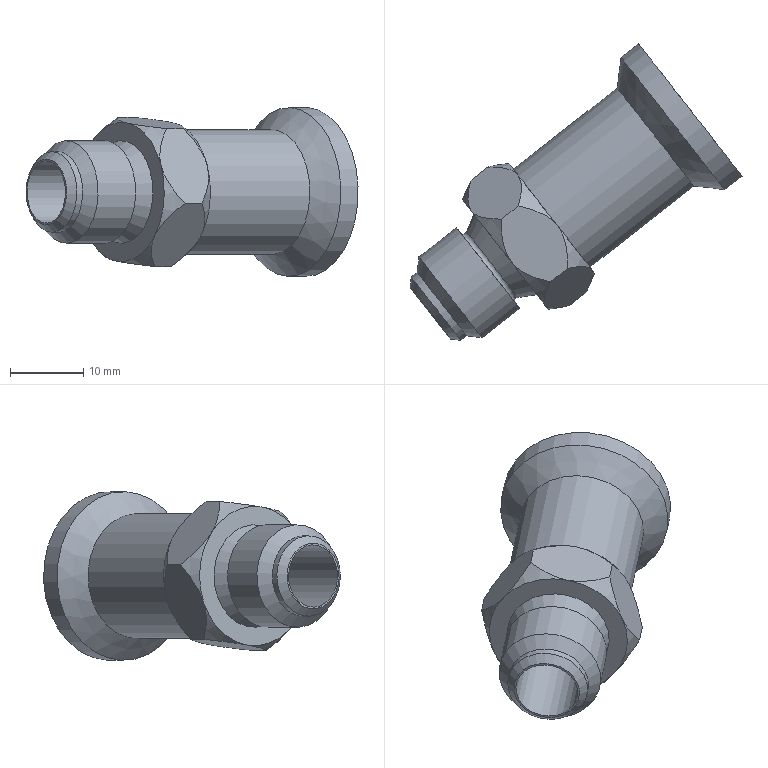Part | NX | features BREP 1 | 1 solid | 35 faces | box 45.311 x 40.485 x 23 mm | volume 6517 mm3 | cone 17 | plane 11 | cylinder 6 | torus 1 | commonest cylinder face diameters 8.5 x1 11 x1 12.5 x1 14 x1 17 x1 23 x1
STEP:
#1=CARTESIAN_POINT('',(-0.7107,91.095,-108.342));
#2=VERTEX_POINT('',#1);
#3=CARTESIAN_POINT('',(-6.134,98.036,-111.901));
#4=VERTEX_POINT('',#3);
#5=CARTESIAN_POINT('',(-1.525,92.137,-117.75));
#6=DIRECTION('',(-0.788,-0.6157,0.));
#7=DIRECTION('',(0.379,-0.4851,0.788));
#8=AXIS2_PLACEMENT_3D('',#5,#6,#7);
#9=CIRCLE('',#8,9.5);
#10=EDGE_CURVE('',#2,#4,#9,.T.);
#11=ORIENTED_EDGE('',*,*,#10,.F.);
#12=CARTESIAN_POINT('',(3.898,85.196,-114.191));
#13=VERTEX_POINT('',#12);
#14=CARTESIAN_POINT('',(-1.525,92.137,-117.75));
#15=DIRECTION('',(-0.788,-0.6157,0.));
#16=DIRECTION('',(0.379,-0.4851,0.788));
#17=AXIS2_PLACEMENT_3D('',#14,#15,#16);
#18=CIRCLE('',#17,9.5);
#19=EDGE_CURVE('',#13,#2,#18,.T.);
#20=ORIENTED_EDGE('',*,*,#19,.F.);
#21=CARTESIAN_POINT('',(3.084,86.238,-123.599));
#22=VERTEX_POINT('',#21);
#23=CARTESIAN_POINT('',(-1.525,92.137,-117.75));
#24=DIRECTION('',(-0.788,-0.6157,0.));
#25=DIRECTION('',(0.379,-0.4851,0.788));
#26=AXIS2_PLACEMENT_3D('',#23,#24,#25);
#27=CIRCLE('',#26,9.5);
#28=EDGE_CURVE('',#22,#13,#27,.T.);
#29=ORIENTED_EDGE('',*,*,#28,.F.);
#30=CARTESIAN_POINT('',(-2.339,93.179,-127.158));
#31=VERTEX_POINT('',#30);
#32=CARTESIAN_POINT('',(-1.525,92.137,-117.75));
#33=DIRECTION('',(-0.788,-0.6157,0.));
#34=DIRECTION('',(0.379,-0.4851,0.788));
#35=AXIS2_PLACEMENT_3D('',#32,#33,#34);
#36=CIRCLE('',#35,9.5);
#37=EDGE_CURVE('',#31,#22,#36,.T.);
#38=ORIENTED_EDGE('',*,*,#37,.F.);
#39=CARTESIAN_POINT('',(-6.948,99.078,-121.309));
#40=VERTEX_POINT('',#39);
#41=CARTESIAN_POINT('',(-1.525,92.137,-117.75));
#42=DIRECTION('',(-0.788,-0.6157,0.));
#43=DIRECTION('',(0.379,-0.4851,0.788));
#44=AXIS2_PLACEMENT_3D('',#41,#42,#43);
#45=CIRCLE('',#44,9.5);
#46=EDGE_CURVE('',#40,#31,#45,.T.);
#47=ORIENTED_EDGE('',*,*,#46,.F.);
#48=CARTESIAN_POINT('',(-1.525,92.137,-117.75));
#49=DIRECTION('',(0.788,0.6157,0.));
#50=DIRECTION('',(-0.379,0.4851,-0.788));
#51=AXIS2_PLACEMENT_3D('',#48,#49,#50);
#52=CIRCLE('',#51,9.5);
#53=EDGE_CURVE('',#40,#4,#52,.T.);
#54=ORIENTED_EDGE('',*,*,#53,.T.);
#55=EDGE_LOOP('',(#11,#20,#29,#38,#47,#54));
#56=FACE_BOUND('',#55,.T.);
#57=CARTESIAN_POINT('',(1.697,88.013,-111.052));
#58=VERTEX_POINT('',#57);
#59=CARTESIAN_POINT('',(-1.525,92.137,-117.75));
#60=DIRECTION('',(0.788,0.6157,0.));
#61=DIRECTION('',(0.379,-0.4851,0.788));
#62=AXIS2_PLACEMENT_3D('',#59,#60,#61);
#63=CIRCLE('',#62,8.5);
#64=EDGE_CURVE('',#58,#58,#63,.T.);
#65=ORIENTED_EDGE('',*,*,#64,.F.);
#66=EDGE_LOOP('',(#65));
#67=FACE_BOUND('',#66,.T.);
#68=CARTESIAN_POINT('',(0.1033,90.053,-98.935));
#69=DIRECTION('',(-0.788,-0.6157,0.));
#70=DIRECTION('',(-0.379,0.4851,-0.788));
#71=AXIS2_PLACEMENT_3D('',#68,#69,#70);
#72=PLANE('',#71);
#73=ADVANCED_FACE('',(#56,#67),#72,.F.);
#74=CARTESIAN_POINT('',(-2.406,80.271,-114.191));
#75=VERTEX_POINT('',#74);
#76=CARTESIAN_POINT('',(-7.015,86.17,-108.342));
#77=VERTEX_POINT('',#76);
#78=CARTESIAN_POINT('',(-7.829,87.212,-117.75));
#79=DIRECTION('',(-0.788,-0.6157,0.));
#80=DIRECTION('',(0.379,-0.4851,0.788));
#81=AXIS2_PLACEMENT_3D('',#78,#79,#80);
#82=CIRCLE('',#81,9.5);
#83=EDGE_CURVE('',#75,#77,#82,.T.);
#84=ORIENTED_EDGE('',*,*,#83,.T.);
#85=CARTESIAN_POINT('',(-12.438,93.111,-111.901));
#86=VERTEX_POINT('',#85);
#87=CARTESIAN_POINT('',(-7.829,87.212,-117.75));
#88=DIRECTION('',(-0.788,-0.6157,0.));
#89=DIRECTION('',(0.379,-0.4851,0.788));
#90=AXIS2_PLACEMENT_3D('',#87,#88,#89);
#91=CIRCLE('',#90,9.5);
#92=EDGE_CURVE('',#77,#86,#91,.T.);
#93=ORIENTED_EDGE('',*,*,#92,.T.);
#94=CARTESIAN_POINT('',(-13.252,94.153,-121.309));
#95=VERTEX_POINT('',#94);
#96=CARTESIAN_POINT('',(-7.829,87.212,-117.75));
#97=DIRECTION('',(-0.788,-0.6157,0.));
#98=DIRECTION('',(0.379,-0.4851,0.788));
#99=AXIS2_PLACEMENT_3D('',#96,#97,#98);
#100=CIRCLE('',#99,9.5);
#101=EDGE_CURVE('',#86,#95,#100,.T.);
#102=ORIENTED_EDGE('',*,*,#101,.T.);
#103=CARTESIAN_POINT('',(-8.643,88.254,-127.158));
#104=VERTEX_POINT('',#103);
#105=CARTESIAN_POINT('',(-7.829,87.212,-117.75));
#106=DIRECTION('',(-0.788,-0.6157,0.));
#107=DIRECTION('',(0.379,-0.4851,0.788));
#108=AXIS2_PLACEMENT_3D('',#105,#106,#107);
#109=CIRCLE('',#108,9.5);
#110=EDGE_CURVE('',#95,#104,#109,.T.);
#111=ORIENTED_EDGE('',*,*,#110,.T.);
#112=CARTESIAN_POINT('',(-3.22,81.313,-123.599));
#113=VERTEX_POINT('',#112);
#114=CARTESIAN_POINT('',(-7.829,87.212,-117.75));
#115=DIRECTION('',(-0.788,-0.6157,0.));
#116=DIRECTION('',(0.379,-0.4851,0.788));
#117=AXIS2_PLACEMENT_3D('',#114,#115,#116);
#118=CIRCLE('',#117,9.5);
#119=EDGE_CURVE('',#104,#113,#118,.T.);
#120=ORIENTED_EDGE('',*,*,#119,.T.);
#121=CARTESIAN_POINT('',(-7.829,87.212,-117.75));
#122=DIRECTION('',(-0.788,-0.6157,0.));
#123=DIRECTION('',(0.379,-0.4851,0.788));
#124=AXIS2_PLACEMENT_3D('',#121,#122,#123);
#125=CIRCLE('',#124,9.5);
#126=EDGE_CURVE('',#113,#75,#125,.T.);
#127=ORIENTED_EDGE('',*,*,#126,.T.);
#128=EDGE_LOOP('',(#84,#93,#102,#111,#120,#127));
#129=FACE_BOUND('',#128,.T.);
#130=CARTESIAN_POINT('',(-10.482,90.608,-123.266));
#131=VERTEX_POINT('',#130);
#132=CARTESIAN_POINT('',(-7.829,87.212,-117.75));
#133=DIRECTION('',(0.788,0.6157,0.));
#134=DIRECTION('',(-0.379,0.4851,-0.788));
#135=AXIS2_PLACEMENT_3D('',#132,#133,#134);
#136=CIRCLE('',#135,7.);
#137=EDGE_CURVE('',#131,#131,#136,.T.);
#138=ORIENTED_EDGE('',*,*,#137,.T.);
#139=EDGE_LOOP('',(#138));
#140=FACE_BOUND('',#139,.T.);
#141=CARTESIAN_POINT('',(-6.201,85.128,-98.935));
#142=DIRECTION('',(-0.788,-0.6157,0.));
#143=DIRECTION('',(-0.379,0.4851,-0.788));
#144=AXIS2_PLACEMENT_3D('',#141,#142,#143);
#145=PLANE('',#144);
#146=ADVANCED_FACE('',(#129,#140),#145,.T.);
#147=CARTESIAN_POINT('',(0.865,80.219,-119.277));
#148=VERTEX_POINT('',#147);
#149=CARTESIAN_POINT('',(0.865,80.219,-119.277));
#150=CARTESIAN_POINT('',(0.1526,80.033,-118.553));
#151=CARTESIAN_POINT('',(-1.199,79.757,-117.033));
#152=CARTESIAN_POINT('',(-2.165,79.963,-115.158));
#153=CARTESIAN_POINT('',(-2.406,80.271,-114.191));
#154=B_SPLINE_CURVE_WITH_KNOTS('',3,(#149,#150,#151,#152,#153),.UNSPECIFIED.,.F.,.F.,(4,1,4),(0.,0.003069,0.006138),.UNSPECIFIED.);
#155=EDGE_CURVE('',#148,#75,#154,.T.);
#156=ORIENTED_EDGE('',*,*,#155,.F.);
#157=CARTESIAN_POINT('',(3.157,82.01,-119.277));
#158=VERTEX_POINT('',#157);
#159=CARTESIAN_POINT('',(-1.141,78.652,-119.277));
#160=DIRECTION('',(0.788,0.6157,0.));
#161=VECTOR('',#160,1000.);
#162=LINE('',#159,#161);
#163=EDGE_CURVE('',#148,#158,#162,.T.);
#164=ORIENTED_EDGE('',*,*,#163,.T.);
#165=CARTESIAN_POINT('',(3.898,85.196,-114.191));
#166=CARTESIAN_POINT('',(4.139,84.888,-115.159));
#167=CARTESIAN_POINT('',(4.107,83.91,-117.018));
#168=CARTESIAN_POINT('',(3.51,82.657,-118.552));
#169=CARTESIAN_POINT('',(3.157,82.01,-119.277));
#170=B_SPLINE_CURVE_WITH_KNOTS('',3,(#165,#166,#167,#168,#169),.UNSPECIFIED.,.F.,.F.,(4,1,4),(0.,0.003072,0.006144),.UNSPECIFIED.);
#171=EDGE_CURVE('',#13,#158,#170,.T.);
#172=ORIENTED_EDGE('',*,*,#171,.F.);
#173=CARTESIAN_POINT('',(0.6273,85.248,-109.106));
#174=VERTEX_POINT('',#173);
#175=CARTESIAN_POINT('',(0.6273,85.248,-109.106));
#176=CARTESIAN_POINT('',(1.34,85.434,-109.829));
#177=CARTESIAN_POINT('',(2.691,85.71,-111.35));
#178=CARTESIAN_POINT('',(3.658,85.504,-113.224));
#179=CARTESIAN_POINT('',(3.898,85.196,-114.191));
#180=B_SPLINE_CURVE_WITH_KNOTS('',3,(#175,#176,#177,#178,#179),.UNSPECIFIED.,.F.,.F.,(4,1,4),(0.,0.003069,0.006138),.UNSPECIFIED.);
#181=EDGE_CURVE('',#174,#13,#180,.T.);
#182=ORIENTED_EDGE('',*,*,#181,.F.);
#183=CARTESIAN_POINT('',(-1.665,83.457,-109.106));
#184=VERTEX_POINT('',#183);
#185=CARTESIAN_POINT('',(-3.671,81.89,-109.106));
#186=DIRECTION('',(0.788,0.6157,0.));
#187=VECTOR('',#186,1000.);
#188=LINE('',#185,#187);
#189=EDGE_CURVE('',#184,#174,#188,.T.);
#190=ORIENTED_EDGE('',*,*,#189,.F.);
#191=CARTESIAN_POINT('',(-2.406,80.271,-114.191));
#192=CARTESIAN_POINT('',(-2.647,80.579,-113.224));
#193=CARTESIAN_POINT('',(-2.615,81.557,-111.365));
#194=CARTESIAN_POINT('',(-2.018,82.81,-109.83));
#195=CARTESIAN_POINT('',(-1.665,83.457,-109.106));
#196=B_SPLINE_CURVE_WITH_KNOTS('',3,(#191,#192,#193,#194,#195),.UNSPECIFIED.,.F.,.F.,(4,1,4),(0.,0.003072,0.006144),.UNSPECIFIED.);
#197=EDGE_CURVE('',#75,#184,#196,.T.);
#198=ORIENTED_EDGE('',*,*,#197,.F.);
#199=EDGE_LOOP('',(#156,#164,#172,#182,#190,#198));
#200=FACE_BOUND('',#199,.T.);
#201=CARTESIAN_POINT('',(-1.141,78.652,-119.277));
#202=DIRECTION('',(-0.5708,0.7306,-0.3746));
#203=DIRECTION('',(-0.2306,0.2952,0.9272));
#204=AXIS2_PLACEMENT_3D('',#201,#202,#203);
#205=PLANE('',#204);
#206=ADVANCED_FACE('',(#200),#205,.F.);
#207=CARTESIAN_POINT('',(-1.665,83.457,-109.106));
#208=CARTESIAN_POINT('',(-2.673,83.65,-108.997));
#209=CARTESIAN_POINT('',(-4.646,84.169,-108.769));
#210=CARTESIAN_POINT('',(-6.379,85.356,-108.488));
#211=CARTESIAN_POINT('',(-7.015,86.17,-108.342));
#212=B_SPLINE_CURVE_WITH_KNOTS('',3,(#207,#208,#209,#210,#211),.UNSPECIFIED.,.F.,.F.,(4,1,4),(0.,0.003069,0.006138),.UNSPECIFIED.);
#213=EDGE_CURVE('',#184,#77,#212,.T.);
#214=ORIENTED_EDGE('',*,*,#213,.F.);
#215=ORIENTED_EDGE('',*,*,#189,.T.);
#216=CARTESIAN_POINT('',(-0.7107,91.095,-108.342));
#217=CARTESIAN_POINT('',(-0.0745,90.281,-108.488));
#218=CARTESIAN_POINT('',(0.6537,88.33,-108.767));
#219=CARTESIAN_POINT('',(0.6842,86.274,-108.997));
#220=CARTESIAN_POINT('',(0.6273,85.248,-109.106));
#221=B_SPLINE_CURVE_WITH_KNOTS('',3,(#216,#217,#218,#219,#220),.UNSPECIFIED.,.F.,.F.,(4,1,4),(0.,0.003072,0.006144),.UNSPECIFIED.);
#222=EDGE_CURVE('',#2,#174,#221,.T.);
#223=ORIENTED_EDGE('',*,*,#222,.F.);
#224=CARTESIAN_POINT('',(-6.061,93.808,-107.579));
#225=VERTEX_POINT('',#224);
#226=CARTESIAN_POINT('',(-6.061,93.808,-107.579));
#227=CARTESIAN_POINT('',(-5.053,93.615,-107.688));
#228=CARTESIAN_POINT('',(-3.079,93.096,-107.916));
#229=CARTESIAN_POINT('',(-1.347,91.909,-108.197));
#230=CARTESIAN_POINT('',(-0.7107,91.095,-108.342));
#231=B_SPLINE_CURVE_WITH_KNOTS('',3,(#226,#227,#228,#229,#230),.UNSPECIFIED.,.F.,.F.,(4,1,4),(0.,0.003069,0.006138),.UNSPECIFIED.);
#232=EDGE_CURVE('',#225,#2,#231,.T.);
#233=ORIENTED_EDGE('',*,*,#232,.F.);
#234=CARTESIAN_POINT('',(-8.353,92.017,-107.579));
#235=VERTEX_POINT('',#234);
#236=CARTESIAN_POINT('',(-10.359,90.45,-107.579));
#237=DIRECTION('',(0.788,0.6157,0.));
#238=VECTOR('',#237,1000.);
#239=LINE('',#236,#238);
#240=EDGE_CURVE('',#235,#225,#239,.T.);
#241=ORIENTED_EDGE('',*,*,#240,.F.);
#242=CARTESIAN_POINT('',(-7.015,86.17,-108.342));
#243=CARTESIAN_POINT('',(-7.651,86.984,-108.197));
#244=CARTESIAN_POINT('',(-8.379,88.935,-107.918));
#245=CARTESIAN_POINT('',(-8.41,90.991,-107.688));
#246=CARTESIAN_POINT('',(-8.353,92.017,-107.579));
#247=B_SPLINE_CURVE_WITH_KNOTS('',3,(#242,#243,#244,#245,#246),.UNSPECIFIED.,.F.,.F.,(4,1,4),(0.,0.003072,0.006144),.UNSPECIFIED.);
#248=EDGE_CURVE('',#77,#235,#247,.T.);
#249=ORIENTED_EDGE('',*,*,#248,.F.);
#250=EDGE_LOOP('',(#214,#215,#223,#233,#241,#249));
#251=FACE_BOUND('',#250,.T.);
#252=CARTESIAN_POINT('',(-3.671,81.89,-109.106));
#253=DIRECTION('',(-0.08568,0.1097,-0.9903));
#254=DIRECTION('',(-0.6097,0.7803,0.1392));
#255=AXIS2_PLACEMENT_3D('',#252,#253,#254);
#256=PLANE('',#255);
#257=ADVANCED_FACE('',(#251),#256,.F.);
#258=CARTESIAN_POINT('',(-8.353,92.017,-107.579));
#259=CARTESIAN_POINT('',(-9.181,91.98,-108.194));
#260=CARTESIAN_POINT('',(-10.776,92.015,-109.486));
#261=CARTESIAN_POINT('',(-12.042,92.605,-111.079));
#262=CARTESIAN_POINT('',(-12.438,93.111,-111.901));
#263=B_SPLINE_CURVE_WITH_KNOTS('',3,(#258,#259,#260,#261,#262),.UNSPECIFIED.,.F.,.F.,(4,1,4),(0.,0.003069,0.006138),.UNSPECIFIED.);
#264=EDGE_CURVE('',#235,#86,#263,.T.);
#265=ORIENTED_EDGE('',*,*,#264,.F.);
#266=ORIENTED_EDGE('',*,*,#240,.T.);
#267=CARTESIAN_POINT('',(-6.134,98.036,-111.901));
#268=CARTESIAN_POINT('',(-5.738,97.53,-111.079));
#269=CARTESIAN_POINT('',(-5.472,96.171,-109.499));
#270=CARTESIAN_POINT('',(-5.823,94.604,-108.195));
#271=CARTESIAN_POINT('',(-6.061,93.808,-107.579));
#272=B_SPLINE_CURVE_WITH_KNOTS('',3,(#267,#268,#269,#270,#271),.UNSPECIFIED.,.F.,.F.,(4,1,4),(0.,0.003072,0.006144),.UNSPECIFIED.);
#273=EDGE_CURVE('',#4,#225,#272,.T.);
#274=ORIENTED_EDGE('',*,*,#273,.F.);
#275=CARTESIAN_POINT('',(-10.218,99.13,-116.223));
#276=VERTEX_POINT('',#275);
#277=CARTESIAN_POINT('',(-10.218,99.13,-116.223));
#278=CARTESIAN_POINT('',(-9.39,99.167,-115.609));
#279=CARTESIAN_POINT('',(-7.796,99.132,-114.316));
#280=CARTESIAN_POINT('',(-6.529,98.542,-112.723));
#281=CARTESIAN_POINT('',(-6.134,98.036,-111.901));
#282=B_SPLINE_CURVE_WITH_KNOTS('',3,(#277,#278,#279,#280,#281),.UNSPECIFIED.,.F.,.F.,(4,1,4),(0.,0.003069,0.006138),.UNSPECIFIED.);
#283=EDGE_CURVE('',#276,#4,#282,.T.);
#284=ORIENTED_EDGE('',*,*,#283,.F.);
#285=CARTESIAN_POINT('',(-12.511,97.339,-116.223));
#286=VERTEX_POINT('',#285);
#287=CARTESIAN_POINT('',(-14.517,95.772,-116.223));
#288=DIRECTION('',(0.788,0.6157,0.));
#289=VECTOR('',#288,1000.);
#290=LINE('',#287,#289);
#291=EDGE_CURVE('',#286,#276,#290,.T.);
#292=ORIENTED_EDGE('',*,*,#291,.F.);
#293=CARTESIAN_POINT('',(-12.438,93.111,-111.901));
#294=CARTESIAN_POINT('',(-12.833,93.617,-112.724));
#295=CARTESIAN_POINT('',(-13.099,94.976,-114.303));
#296=CARTESIAN_POINT('',(-12.748,96.543,-115.608));
#297=CARTESIAN_POINT('',(-12.511,97.339,-116.223));
#298=B_SPLINE_CURVE_WITH_KNOTS('',3,(#293,#294,#295,#296,#297),.UNSPECIFIED.,.F.,.F.,(4,1,4),(0.,0.003072,0.006144),.UNSPECIFIED.);
#299=EDGE_CURVE('',#86,#286,#298,.T.);
#300=ORIENTED_EDGE('',*,*,#299,.F.);
#301=EDGE_LOOP('',(#265,#266,#274,#284,#292,#300));
#302=FACE_BOUND('',#301,.T.);
#303=CARTESIAN_POINT('',(-10.359,90.45,-107.579));
#304=DIRECTION('',(0.4851,-0.621,-0.6157));
#305=DIRECTION('',(-0.788,-0.6157,0.));
#306=AXIS2_PLACEMENT_3D('',#303,#304,#305);
#307=PLANE('',#306);
#308=ADVANCED_FACE('',(#302),#307,.F.);
#309=CARTESIAN_POINT('',(-12.511,97.339,-116.223));
#310=CARTESIAN_POINT('',(-12.863,96.693,-116.947));
#311=CARTESIAN_POINT('',(-13.458,95.448,-118.467));
#312=CARTESIAN_POINT('',(-13.492,94.461,-120.342));
#313=CARTESIAN_POINT('',(-13.252,94.153,-121.309));
#314=B_SPLINE_CURVE_WITH_KNOTS('',3,(#309,#310,#311,#312,#313),.UNSPECIFIED.,.F.,.F.,(4,1,4),(0.,0.003069,0.006138),.UNSPECIFIED.);
#315=EDGE_CURVE('',#286,#95,#314,.T.);
#316=ORIENTED_EDGE('',*,*,#315,.F.);
#317=ORIENTED_EDGE('',*,*,#291,.T.);
#318=CARTESIAN_POINT('',(-6.948,99.078,-121.309));
#319=CARTESIAN_POINT('',(-7.188,99.386,-120.341));
#320=CARTESIAN_POINT('',(-8.145,99.592,-118.482));
#321=CARTESIAN_POINT('',(-9.505,99.316,-116.948));
#322=CARTESIAN_POINT('',(-10.218,99.13,-116.223));
#323=B_SPLINE_CURVE_WITH_KNOTS('',3,(#318,#319,#320,#321,#322),.UNSPECIFIED.,.F.,.F.,(4,1,4),(0.,0.003072,0.006144),.UNSPECIFIED.);
#324=EDGE_CURVE('',#40,#276,#323,.T.);
#325=ORIENTED_EDGE('',*,*,#324,.F.);
#326=CARTESIAN_POINT('',(-7.689,95.892,-126.394));
#327=VERTEX_POINT('',#326);
#328=CARTESIAN_POINT('',(-7.689,95.892,-126.394));
#329=CARTESIAN_POINT('',(-7.336,96.538,-125.671));
#330=CARTESIAN_POINT('',(-6.741,97.783,-124.15));
#331=CARTESIAN_POINT('',(-6.707,98.77,-122.276));
#332=CARTESIAN_POINT('',(-6.948,99.078,-121.309));
#333=B_SPLINE_CURVE_WITH_KNOTS('',3,(#328,#329,#330,#331,#332),.UNSPECIFIED.,.F.,.F.,(4,1,4),(0.,0.003069,0.006138),.UNSPECIFIED.);
#334=EDGE_CURVE('',#327,#40,#333,.T.);
#335=ORIENTED_EDGE('',*,*,#334,.F.);
#336=CARTESIAN_POINT('',(-9.981,94.101,-126.394));
#337=VERTEX_POINT('',#336);
#338=CARTESIAN_POINT('',(-11.987,92.534,-126.394));
#339=DIRECTION('',(0.788,0.6157,0.));
#340=VECTOR('',#339,1000.);
#341=LINE('',#338,#340);
#342=EDGE_CURVE('',#337,#327,#341,.T.);
#343=ORIENTED_EDGE('',*,*,#342,.F.);
#344=CARTESIAN_POINT('',(-13.252,94.153,-121.309));
#345=CARTESIAN_POINT('',(-13.011,93.845,-122.276));
#346=CARTESIAN_POINT('',(-12.055,93.639,-124.135));
#347=CARTESIAN_POINT('',(-10.694,93.915,-125.67));
#348=CARTESIAN_POINT('',(-9.981,94.101,-126.394));
#349=B_SPLINE_CURVE_WITH_KNOTS('',3,(#344,#345,#346,#347,#348),.UNSPECIFIED.,.F.,.F.,(4,1,4),(0.,0.003072,0.006144),.UNSPECIFIED.);
#350=EDGE_CURVE('',#95,#337,#349,.T.);
#351=ORIENTED_EDGE('',*,*,#350,.F.);
#352=EDGE_LOOP('',(#316,#317,#325,#335,#343,#351));
#353=FACE_BOUND('',#352,.T.);
#354=CARTESIAN_POINT('',(-14.517,95.772,-116.223));
#355=DIRECTION('',(0.5708,-0.7306,0.3746));
#356=DIRECTION('',(0.2306,-0.2952,-0.9272));
#357=AXIS2_PLACEMENT_3D('',#354,#355,#356);
#358=PLANE('',#357);
#359=ADVANCED_FACE('',(#353),#358,.F.);
#360=CARTESIAN_POINT('',(-9.981,94.101,-126.394));
#361=CARTESIAN_POINT('',(-10.038,93.076,-126.503));
#362=CARTESIAN_POINT('',(-10.011,91.036,-126.731));
#363=CARTESIAN_POINT('',(-9.279,89.068,-127.012));
#364=CARTESIAN_POINT('',(-8.643,88.254,-127.158));
#365=B_SPLINE_CURVE_WITH_KNOTS('',3,(#360,#361,#362,#363,#364),.UNSPECIFIED.,.F.,.F.,(4,1,4),(0.,0.003069,0.006138),.UNSPECIFIED.);
#366=EDGE_CURVE('',#337,#104,#365,.T.);
#367=ORIENTED_EDGE('',*,*,#366,.F.);
#368=ORIENTED_EDGE('',*,*,#342,.T.);
#369=CARTESIAN_POINT('',(-2.339,93.179,-127.158));
#370=CARTESIAN_POINT('',(-2.975,93.993,-127.012));
#371=CARTESIAN_POINT('',(-4.691,95.172,-126.733));
#372=CARTESIAN_POINT('',(-6.679,95.699,-126.503));
#373=CARTESIAN_POINT('',(-7.689,95.892,-126.394));
#374=B_SPLINE_CURVE_WITH_KNOTS('',3,(#369,#370,#371,#372,#373),.UNSPECIFIED.,.F.,.F.,(4,1,4),(0.,0.003072,0.006144),.UNSPECIFIED.);
#375=EDGE_CURVE('',#31,#327,#374,.T.);
#376=ORIENTED_EDGE('',*,*,#375,.F.);
#377=CARTESIAN_POINT('',(-1.001,87.332,-127.921));
#378=VERTEX_POINT('',#377);
#379=CARTESIAN_POINT('',(-1.001,87.332,-127.921));
#380=CARTESIAN_POINT('',(-0.9439,88.356,-127.812));
#381=CARTESIAN_POINT('',(-0.9707,90.397,-127.584));
#382=CARTESIAN_POINT('',(-1.703,92.365,-127.303));
#383=CARTESIAN_POINT('',(-2.339,93.179,-127.158));
#384=B_SPLINE_CURVE_WITH_KNOTS('',3,(#379,#380,#381,#382,#383),.UNSPECIFIED.,.F.,.F.,(4,1,4),(0.,0.003069,0.006138),.UNSPECIFIED.);
#385=EDGE_CURVE('',#378,#31,#384,.T.);
#386=ORIENTED_EDGE('',*,*,#385,.F.);
#387=CARTESIAN_POINT('',(-3.293,85.541,-127.921));
#388=VERTEX_POINT('',#387);
#389=CARTESIAN_POINT('',(-5.299,83.974,-127.921));
#390=DIRECTION('',(0.788,0.6157,0.));
#391=VECTOR('',#390,1000.);
#392=LINE('',#389,#391);
#393=EDGE_CURVE('',#388,#378,#392,.T.);
#394=ORIENTED_EDGE('',*,*,#393,.F.);
#395=CARTESIAN_POINT('',(-8.643,88.254,-127.158));
#396=CARTESIAN_POINT('',(-8.007,87.439,-127.303));
#397=CARTESIAN_POINT('',(-6.29,86.261,-127.582));
#398=CARTESIAN_POINT('',(-4.303,85.734,-127.812));
#399=CARTESIAN_POINT('',(-3.293,85.541,-127.921));
#400=B_SPLINE_CURVE_WITH_KNOTS('',3,(#395,#396,#397,#398,#399),.UNSPECIFIED.,.F.,.F.,(4,1,4),(0.,0.003072,0.006144),.UNSPECIFIED.);
#401=EDGE_CURVE('',#104,#388,#400,.T.);
#402=ORIENTED_EDGE('',*,*,#401,.F.);
#403=EDGE_LOOP('',(#367,#368,#376,#386,#394,#402));
#404=FACE_BOUND('',#403,.T.);
#405=CARTESIAN_POINT('',(-11.987,92.534,-126.394));
#406=DIRECTION('',(0.08568,-0.1097,0.9903));
#407=DIRECTION('',(0.6097,-0.7803,-0.1392));
#408=AXIS2_PLACEMENT_3D('',#405,#406,#407);
#409=PLANE('',#408);
#410=ADVANCED_FACE('',(#404),#409,.F.);
#411=CARTESIAN_POINT('',(-3.293,85.541,-127.921));
#412=CARTESIAN_POINT('',(-3.53,84.746,-127.306));
#413=CARTESIAN_POINT('',(-3.881,83.19,-126.014));
#414=CARTESIAN_POINT('',(-3.615,81.819,-124.421));
#415=CARTESIAN_POINT('',(-3.22,81.313,-123.599));
#416=B_SPLINE_CURVE_WITH_KNOTS('',3,(#411,#412,#413,#414,#415),.UNSPECIFIED.,.F.,.F.,(4,1,4),(0.,0.003069,0.006138),.UNSPECIFIED.);
#417=EDGE_CURVE('',#388,#113,#416,.T.);
#418=ORIENTED_EDGE('',*,*,#417,.F.);
#419=ORIENTED_EDGE('',*,*,#393,.T.);
#420=CARTESIAN_POINT('',(3.084,86.238,-123.599));
#421=CARTESIAN_POINT('',(2.689,86.744,-124.421));
#422=CARTESIAN_POINT('',(1.435,87.331,-126.001));
#423=CARTESIAN_POINT('',(-0.1712,87.369,-127.305));
#424=CARTESIAN_POINT('',(-1.001,87.332,-127.921));
#425=B_SPLINE_CURVE_WITH_KNOTS('',3,(#420,#421,#422,#423,#424),.UNSPECIFIED.,.F.,.F.,(4,1,4),(0.,0.003072,0.006144),.UNSPECIFIED.);
#426=EDGE_CURVE('',#22,#378,#425,.T.);
#427=ORIENTED_EDGE('',*,*,#426,.F.);
#428=CARTESIAN_POINT('',(3.157,82.01,-119.277));
#429=CARTESIAN_POINT('',(3.394,82.804,-119.891));
#430=CARTESIAN_POINT('',(3.745,84.36,-121.184));
#431=CARTESIAN_POINT('',(3.48,85.732,-122.777));
#432=CARTESIAN_POINT('',(3.084,86.238,-123.599));
#433=B_SPLINE_CURVE_WITH_KNOTS('',3,(#428,#429,#430,#431,#432),.UNSPECIFIED.,.F.,.F.,(4,1,4),(0.,0.003069,0.006138),.UNSPECIFIED.);
#434=EDGE_CURVE('',#158,#22,#433,.T.);
#435=ORIENTED_EDGE('',*,*,#434,.F.);
#436=ORIENTED_EDGE('',*,*,#163,.F.);
#437=CARTESIAN_POINT('',(-3.22,81.313,-123.599));
#438=CARTESIAN_POINT('',(-2.824,80.806,-122.776));
#439=CARTESIAN_POINT('',(-1.57,80.22,-121.197));
#440=CARTESIAN_POINT('',(0.03551,80.181,-119.892));
#441=CARTESIAN_POINT('',(0.865,80.219,-119.277));
#442=B_SPLINE_CURVE_WITH_KNOTS('',3,(#437,#438,#439,#440,#441),.UNSPECIFIED.,.F.,.F.,(4,1,4),(0.,0.003072,0.006144),.UNSPECIFIED.);
#443=EDGE_CURVE('',#113,#148,#442,.T.);
#444=ORIENTED_EDGE('',*,*,#443,.F.);
#445=EDGE_LOOP('',(#418,#419,#427,#435,#436,#444));
#446=FACE_BOUND('',#445,.T.);
#447=CARTESIAN_POINT('',(-5.299,83.974,-127.921));
#448=DIRECTION('',(-0.4851,0.621,0.6157));
#449=DIRECTION('',(0.379,-0.4851,0.788));
#450=AXIS2_PLACEMENT_3D('',#447,#448,#449);
#451=PLANE('',#450);
#452=ADVANCED_FACE('',(#446),#451,.F.);
#453=ORIENTED_EDGE('',*,*,#222,.T.);
#454=ORIENTED_EDGE('',*,*,#181,.T.);
#455=ORIENTED_EDGE('',*,*,#19,.T.);
#456=EDGE_LOOP('',(#453,#454,#455));
#457=FACE_BOUND('',#456,.T.);
#458=CARTESIAN_POINT('',(-1.525,92.137,-117.75));
#459=DIRECTION('',(-0.788,-0.6157,0.));
#460=DIRECTION('',(0.379,-0.4851,0.788));
#461=AXIS2_PLACEMENT_3D('',#458,#459,#460);
#462=CONICAL_SURFACE('',#461,9.5,0.5236);
#463=ADVANCED_FACE('',(#457),#462,.T.);
#464=ORIENTED_EDGE('',*,*,#171,.T.);
#465=ORIENTED_EDGE('',*,*,#434,.T.);
#466=ORIENTED_EDGE('',*,*,#28,.T.);
#467=EDGE_LOOP('',(#464,#465,#466));
#468=FACE_BOUND('',#467,.T.);
#469=CARTESIAN_POINT('',(-1.525,92.137,-117.75));
#470=DIRECTION('',(-0.788,-0.6157,0.));
#471=DIRECTION('',(0.379,-0.4851,0.788));
#472=AXIS2_PLACEMENT_3D('',#469,#470,#471);
#473=CONICAL_SURFACE('',#472,9.5,0.5236);
#474=ADVANCED_FACE('',(#468),#473,.T.);
#475=ORIENTED_EDGE('',*,*,#385,.T.);
#476=ORIENTED_EDGE('',*,*,#37,.T.);
#477=ORIENTED_EDGE('',*,*,#426,.T.);
#478=EDGE_LOOP('',(#475,#476,#477));
#479=FACE_BOUND('',#478,.T.);
#480=CARTESIAN_POINT('',(-1.525,92.137,-117.75));
#481=DIRECTION('',(-0.788,-0.6157,0.));
#482=DIRECTION('',(0.379,-0.4851,0.788));
#483=AXIS2_PLACEMENT_3D('',#480,#481,#482);
#484=CONICAL_SURFACE('',#483,9.5,0.5236);
#485=ADVANCED_FACE('',(#479),#484,.T.);
#486=ORIENTED_EDGE('',*,*,#334,.T.);
#487=ORIENTED_EDGE('',*,*,#46,.T.);
#488=ORIENTED_EDGE('',*,*,#375,.T.);
#489=EDGE_LOOP('',(#486,#487,#488));
#490=FACE_BOUND('',#489,.T.);
#491=CARTESIAN_POINT('',(-1.525,92.137,-117.75));
#492=DIRECTION('',(-0.788,-0.6157,0.));
#493=DIRECTION('',(0.379,-0.4851,0.788));
#494=AXIS2_PLACEMENT_3D('',#491,#492,#493);
#495=CONICAL_SURFACE('',#494,9.5,0.5236);
#496=ADVANCED_FACE('',(#490),#495,.T.);
#497=ORIENTED_EDGE('',*,*,#283,.T.);
#498=ORIENTED_EDGE('',*,*,#53,.F.);
#499=ORIENTED_EDGE('',*,*,#324,.T.);
#500=EDGE_LOOP('',(#497,#498,#499));
#501=FACE_BOUND('',#500,.T.);
#502=CARTESIAN_POINT('',(-1.525,92.137,-117.75));
#503=DIRECTION('',(-0.788,-0.6157,0.));
#504=DIRECTION('',(0.379,-0.4851,0.788));
#505=AXIS2_PLACEMENT_3D('',#502,#503,#504);
#506=CONICAL_SURFACE('',#505,9.5,0.5236);
#507=ADVANCED_FACE('',(#501),#506,.T.);
#508=ORIENTED_EDGE('',*,*,#273,.T.);
#509=ORIENTED_EDGE('',*,*,#232,.T.);
#510=ORIENTED_EDGE('',*,*,#10,.T.);
#511=EDGE_LOOP('',(#508,#509,#510));
#512=FACE_BOUND('',#511,.T.);
#513=CARTESIAN_POINT('',(-1.525,92.137,-117.75));
#514=DIRECTION('',(-0.788,-0.6157,0.));
#515=DIRECTION('',(0.379,-0.4851,0.788));
#516=AXIS2_PLACEMENT_3D('',#513,#514,#515);
#517=CONICAL_SURFACE('',#516,9.5,0.5236);
#518=ADVANCED_FACE('',(#512),#517,.T.);
#519=ORIENTED_EDGE('',*,*,#197,.T.);
#520=ORIENTED_EDGE('',*,*,#213,.T.);
#521=ORIENTED_EDGE('',*,*,#83,.F.);
#522=EDGE_LOOP('',(#519,#520,#521));
#523=FACE_BOUND('',#522,.T.);
#524=CARTESIAN_POINT('',(-7.829,87.212,-117.75));
#525=DIRECTION('',(0.788,0.6157,0.));
#526=DIRECTION('',(-0.379,0.4851,-0.788));
#527=AXIS2_PLACEMENT_3D('',#524,#525,#526);
#528=CONICAL_SURFACE('',#527,9.5,0.5236);
#529=ADVANCED_FACE('',(#523),#528,.T.);
#530=ORIENTED_EDGE('',*,*,#155,.T.);
#531=ORIENTED_EDGE('',*,*,#126,.F.);
#532=ORIENTED_EDGE('',*,*,#443,.T.);
#533=EDGE_LOOP('',(#530,#531,#532));
#534=FACE_BOUND('',#533,.T.);
#535=CARTESIAN_POINT('',(-7.829,87.212,-117.75));
#536=DIRECTION('',(0.788,0.6157,0.));
#537=DIRECTION('',(-0.379,0.4851,-0.788));
#538=AXIS2_PLACEMENT_3D('',#535,#536,#537);
#539=CONICAL_SURFACE('',#538,9.5,0.5236);
#540=ADVANCED_FACE('',(#534),#539,.T.);
#541=ORIENTED_EDGE('',*,*,#401,.T.);
#542=ORIENTED_EDGE('',*,*,#417,.T.);
#543=ORIENTED_EDGE('',*,*,#119,.F.);
#544=EDGE_LOOP('',(#541,#542,#543));
#545=FACE_BOUND('',#544,.T.);
#546=CARTESIAN_POINT('',(-7.829,87.212,-117.75));
#547=DIRECTION('',(0.788,0.6157,0.));
#548=DIRECTION('',(-0.379,0.4851,-0.788));
#549=AXIS2_PLACEMENT_3D('',#546,#547,#548);
#550=CONICAL_SURFACE('',#549,9.5,0.5236);
#551=ADVANCED_FACE('',(#545),#550,.T.);
#552=ORIENTED_EDGE('',*,*,#350,.T.);
#553=ORIENTED_EDGE('',*,*,#366,.T.);
#554=ORIENTED_EDGE('',*,*,#110,.F.);
#555=EDGE_LOOP('',(#552,#553,#554));
#556=FACE_BOUND('',#555,.T.);
#557=CARTESIAN_POINT('',(-7.829,87.212,-117.75));
#558=DIRECTION('',(0.788,0.6157,0.));
#559=DIRECTION('',(-0.379,0.4851,-0.788));
#560=AXIS2_PLACEMENT_3D('',#557,#558,#559);
#561=CONICAL_SURFACE('',#560,9.5,0.5236);
#562=ADVANCED_FACE('',(#556),#561,.T.);
#563=ORIENTED_EDGE('',*,*,#299,.T.);
#564=ORIENTED_EDGE('',*,*,#315,.T.);
#565=ORIENTED_EDGE('',*,*,#101,.F.);
#566=EDGE_LOOP('',(#563,#564,#565));
#567=FACE_BOUND('',#566,.T.);
#568=CARTESIAN_POINT('',(-7.829,87.212,-117.75));
#569=DIRECTION('',(0.788,0.6157,0.));
#570=DIRECTION('',(-0.379,0.4851,-0.788));
#571=AXIS2_PLACEMENT_3D('',#568,#569,#570);
#572=CONICAL_SURFACE('',#571,9.5,0.5236);
#573=ADVANCED_FACE('',(#567),#572,.T.);
#574=ORIENTED_EDGE('',*,*,#248,.T.);
#575=ORIENTED_EDGE('',*,*,#264,.T.);
#576=ORIENTED_EDGE('',*,*,#92,.F.);
#577=EDGE_LOOP('',(#574,#575,#576));
#578=FACE_BOUND('',#577,.T.);
#579=CARTESIAN_POINT('',(-7.829,87.212,-117.75));
#580=DIRECTION('',(0.788,0.6157,0.));
#581=DIRECTION('',(-0.379,0.4851,-0.788));
#582=AXIS2_PLACEMENT_3D('',#579,#580,#581);
#583=CONICAL_SURFACE('',#582,9.5,0.5236);
#584=ADVANCED_FACE('',(#578),#583,.T.);
#585=ORIENTED_EDGE('',*,*,#137,.F.);
#586=EDGE_LOOP('',(#585));
#587=FACE_BOUND('',#586,.T.);
#588=CARTESIAN_POINT('',(-11.772,88.578,-122.235));
#589=VERTEX_POINT('',#588);
#590=CARTESIAN_POINT('',(-9.614,85.817,-117.75));
#591=DIRECTION('',(0.788,0.6157,0.));
#592=DIRECTION('',(-0.379,0.4851,-0.788));
#593=AXIS2_PLACEMENT_3D('',#590,#591,#592);
#594=CIRCLE('',#593,5.692);
#595=EDGE_CURVE('',#589,#589,#594,.T.);
#596=ORIENTED_EDGE('',*,*,#595,.T.);
#597=EDGE_LOOP('',(#596));
#598=FACE_BOUND('',#597,.T.);
#599=CARTESIAN_POINT('',(-9.614,85.817,-117.75));
#600=DIRECTION('',(0.788,0.6157,0.));
#601=DIRECTION('',(0.379,-0.4851,0.788));
#602=AXIS2_PLACEMENT_3D('',#599,#600,#601);
#603=CONICAL_SURFACE('',#602,5.692,0.5236);
#604=ADVANCED_FACE('',(#587,#598),#603,.T.);
#605=ORIENTED_EDGE('',*,*,#595,.F.);
#606=EDGE_LOOP('',(#605));
#607=FACE_BOUND('',#606,.T.);
#608=CARTESIAN_POINT('',(-12.562,88.397,-122.675));
#609=VERTEX_POINT('',#608);
#610=CARTESIAN_POINT('',(-10.193,85.365,-117.75));
#611=DIRECTION('',(0.788,0.6157,0.));
#612=DIRECTION('',(-0.379,0.4851,-0.788));
#613=AXIS2_PLACEMENT_3D('',#610,#611,#612);
#614=CIRCLE('',#613,6.25);
#615=EDGE_CURVE('',#609,#609,#614,.T.);
#616=ORIENTED_EDGE('',*,*,#615,.T.);
#617=EDGE_LOOP('',(#616));
#618=FACE_BOUND('',#617,.T.);
#619=CARTESIAN_POINT('',(-9.811,85.663,-117.75));
#620=DIRECTION('',(0.788,0.6157,0.));
#621=DIRECTION('',(0.379,-0.4851,0.788));
#622=AXIS2_PLACEMENT_3D('',#619,#620,#621);
#623=TOROIDAL_SURFACE('',#622,6.125,0.5);
#624=ADVANCED_FACE('',(#607,#618),#623,.F.);
#625=ORIENTED_EDGE('',*,*,#615,.F.);
#626=EDGE_LOOP('',(#625));
#627=FACE_BOUND('',#626,.T.);
#628=CARTESIAN_POINT('',(-12.846,88.761,-123.266));
#629=VERTEX_POINT('',#628);
#630=CARTESIAN_POINT('',(-10.193,85.365,-117.75));
#631=DIRECTION('',(0.788,0.6157,0.));
#632=DIRECTION('',(-0.379,0.4851,-0.788));
#633=AXIS2_PLACEMENT_3D('',#630,#631,#632);
#634=CIRCLE('',#633,7.);
#635=EDGE_CURVE('',#629,#629,#634,.T.);
#636=ORIENTED_EDGE('',*,*,#635,.T.);
#637=EDGE_LOOP('',(#636));
#638=FACE_BOUND('',#637,.T.);
#639=CARTESIAN_POINT('',(-7.824,82.333,-112.825));
#640=DIRECTION('',(-0.788,-0.6157,0.));
#641=DIRECTION('',(-0.379,0.4851,-0.788));
#642=AXIS2_PLACEMENT_3D('',#639,#640,#641);
#643=PLANE('',#642);
#644=ADVANCED_FACE('',(#627,#638),#643,.F.);
#645=ORIENTED_EDGE('',*,*,#635,.F.);
#646=EDGE_LOOP('',(#645));
#647=FACE_BOUND('',#646,.T.);
#648=CARTESIAN_POINT('',(-17.968,84.759,-123.266));
#649=VERTEX_POINT('',#648);
#650=CARTESIAN_POINT('',(-15.315,81.363,-117.75));
#651=DIRECTION('',(0.788,0.6157,0.));
#652=DIRECTION('',(-0.379,0.4851,-0.788));
#653=AXIS2_PLACEMENT_3D('',#650,#651,#652);
#654=CIRCLE('',#653,7.);
#655=EDGE_CURVE('',#649,#649,#654,.T.);
#656=ORIENTED_EDGE('',*,*,#655,.T.);
#657=EDGE_LOOP('',(#656));
#658=FACE_BOUND('',#657,.T.);
#659=CARTESIAN_POINT('',(36.05,121.494,-117.75));
#660=DIRECTION('',(0.788,0.6157,0.));
#661=DIRECTION('',(0.379,-0.4851,0.788));
#662=AXIS2_PLACEMENT_3D('',#659,#660,#661);
#663=CYLINDRICAL_SURFACE('',#662,7.);
#664=ADVANCED_FACE('',(#647,#658),#663,.T.);
#665=ORIENTED_EDGE('',*,*,#655,.F.);
#666=EDGE_LOOP('',(#665));
#667=FACE_BOUND('',#666,.T.);
#668=CARTESIAN_POINT('',(-18.582,83.108,-122.084));
#669=VERTEX_POINT('',#668);
#670=CARTESIAN_POINT('',(-16.497,80.439,-117.75));
#671=DIRECTION('',(0.788,0.6157,0.));
#672=DIRECTION('',(-0.379,0.4851,-0.788));
#673=AXIS2_PLACEMENT_3D('',#670,#671,#672);
#674=CIRCLE('',#673,5.5);
#675=EDGE_CURVE('',#669,#669,#674,.T.);
#676=ORIENTED_EDGE('',*,*,#675,.T.);
#677=EDGE_LOOP('',(#676));
#678=FACE_BOUND('',#677,.T.);
#679=CARTESIAN_POINT('',(-16.497,80.439,-117.75));
#680=DIRECTION('',(0.788,0.6157,0.));
#681=DIRECTION('',(0.379,-0.4851,0.788));
#682=AXIS2_PLACEMENT_3D('',#679,#680,#681);
#683=CONICAL_SURFACE('',#682,5.5,0.7854);
#684=ADVANCED_FACE('',(#667,#678),#683,.T.);
#685=ORIENTED_EDGE('',*,*,#675,.F.);
#686=EDGE_LOOP('',(#685));
#687=FACE_BOUND('',#686,.T.);
#688=CARTESIAN_POINT('',(-19.37,82.492,-122.084));
#689=VERTEX_POINT('',#688);
#690=CARTESIAN_POINT('',(-17.285,79.824,-117.75));
#691=DIRECTION('',(0.788,0.6157,0.));
#692=DIRECTION('',(-0.379,0.4851,-0.788));
#693=AXIS2_PLACEMENT_3D('',#690,#691,#692);
#694=CIRCLE('',#693,5.5);
#695=EDGE_CURVE('',#689,#689,#694,.T.);
#696=ORIENTED_EDGE('',*,*,#695,.T.);
#697=EDGE_LOOP('',(#696));
#698=FACE_BOUND('',#697,.T.);
#699=CARTESIAN_POINT('',(36.05,121.494,-117.75));
#700=DIRECTION('',(0.788,0.6157,0.));
#701=DIRECTION('',(0.379,-0.4851,0.788));
#702=AXIS2_PLACEMENT_3D('',#699,#700,#701);
#703=CYLINDRICAL_SURFACE('',#702,5.5);
#704=ADVANCED_FACE('',(#687,#698),#703,.T.);
#705=ORIENTED_EDGE('',*,*,#695,.F.);
#706=EDGE_LOOP('',(#705));
#707=FACE_BOUND('',#706,.T.);
#708=CARTESIAN_POINT('',(-19.779,81.391,-121.296));
#709=VERTEX_POINT('',#708);
#710=CARTESIAN_POINT('',(-18.073,79.208,-117.75));
#711=DIRECTION('',(0.788,0.6157,0.));
#712=DIRECTION('',(-0.379,0.4851,-0.788));
#713=AXIS2_PLACEMENT_3D('',#710,#711,#712);
#714=CIRCLE('',#713,4.5);
#715=EDGE_CURVE('',#709,#709,#714,.T.);
#716=ORIENTED_EDGE('',*,*,#715,.T.);
#717=EDGE_LOOP('',(#716));
#718=FACE_BOUND('',#717,.T.);
#719=CARTESIAN_POINT('',(-18.073,79.208,-117.75));
#720=DIRECTION('',(0.788,0.6157,0.));
#721=DIRECTION('',(0.379,-0.4851,0.788));
#722=AXIS2_PLACEMENT_3D('',#719,#720,#721);
#723=CONICAL_SURFACE('',#722,4.5,0.7854);
#724=ADVANCED_FACE('',(#707,#718),#723,.T.);
#725=CARTESIAN_POINT('',(-16.462,77.146,-114.401));
#726=VERTEX_POINT('',#725);
#727=CARTESIAN_POINT('',(-18.073,79.208,-117.75));
#728=DIRECTION('',(-0.788,-0.6157,0.));
#729=DIRECTION('',(0.379,-0.4851,0.788));
#730=AXIS2_PLACEMENT_3D('',#727,#728,#729);
#731=CIRCLE('',#730,4.25);
#732=EDGE_CURVE('',#726,#726,#731,.T.);
#733=ORIENTED_EDGE('',*,*,#732,.F.);
#734=EDGE_LOOP('',(#733));
#735=FACE_BOUND('',#734,.T.);
#736=ORIENTED_EDGE('',*,*,#715,.F.);
#737=EDGE_LOOP('',(#736));
#738=FACE_BOUND('',#737,.T.);
#739=CARTESIAN_POINT('',(-16.367,77.025,-114.204));
#740=DIRECTION('',(0.788,0.6157,0.));
#741=DIRECTION('',(0.379,-0.4851,0.788));
#742=AXIS2_PLACEMENT_3D('',#739,#740,#741);
#743=PLANE('',#742);
#744=ADVANCED_FACE('',(#735,#738),#743,.F.);
#745=CARTESIAN_POINT('',(9.438,107.343,-124.448));
#746=VERTEX_POINT('',#745);
#747=CARTESIAN_POINT('',(12.659,103.219,-117.75));
#748=DIRECTION('',(0.788,0.6157,0.));
#749=DIRECTION('',(-0.379,0.4851,-0.788));
#750=AXIS2_PLACEMENT_3D('',#747,#748,#749);
#751=CIRCLE('',#750,8.5);
#752=EDGE_CURVE('',#746,#746,#751,.T.);
#753=ORIENTED_EDGE('',*,*,#752,.F.);
#754=EDGE_LOOP('',(#753));
#755=FACE_BOUND('',#754,.T.);
#756=ORIENTED_EDGE('',*,*,#64,.T.);
#757=EDGE_LOOP('',(#756));
#758=FACE_BOUND('',#757,.T.);
#759=CARTESIAN_POINT('',(36.05,121.494,-117.75));
#760=DIRECTION('',(0.788,0.6157,0.));
#761=DIRECTION('',(0.379,-0.4851,0.788));
#762=AXIS2_PLACEMENT_3D('',#759,#760,#761);
#763=CYLINDRICAL_SURFACE('',#762,8.5);
#764=ADVANCED_FACE('',(#755,#758),#763,.T.);
#765=CARTESIAN_POINT('',(10.665,110.645,-126.812));
#766=VERTEX_POINT('',#765);
#767=CARTESIAN_POINT('',(15.024,105.066,-117.75));
#768=DIRECTION('',(0.788,0.6157,0.));
#769=DIRECTION('',(-0.379,0.4851,-0.788));
#770=AXIS2_PLACEMENT_3D('',#767,#768,#769);
#771=CIRCLE('',#770,11.5);
#772=EDGE_CURVE('',#766,#766,#771,.T.);
#773=ORIENTED_EDGE('',*,*,#772,.F.);
#774=EDGE_LOOP('',(#773));
#775=FACE_BOUND('',#774,.T.);
#776=ORIENTED_EDGE('',*,*,#752,.T.);
#777=EDGE_LOOP('',(#776));
#778=FACE_BOUND('',#777,.T.);
#779=CARTESIAN_POINT('',(12.659,103.219,-117.75));
#780=DIRECTION('',(0.788,0.6157,0.));
#781=DIRECTION('',(0.379,-0.4851,0.788));
#782=AXIS2_PLACEMENT_3D('',#779,#780,#781);
#783=CONICAL_SURFACE('',#782,8.5,0.7854);
#784=ADVANCED_FACE('',(#775,#778),#783,.T.);
#785=CARTESIAN_POINT('',(13.029,112.492,-126.812));
#786=VERTEX_POINT('',#785);
#787=CARTESIAN_POINT('',(17.388,106.913,-117.75));
#788=DIRECTION('',(0.788,0.6157,0.));
#789=DIRECTION('',(-0.379,0.4851,-0.788));
#790=AXIS2_PLACEMENT_3D('',#787,#788,#789);
#791=CIRCLE('',#790,11.5);
#792=EDGE_CURVE('',#786,#786,#791,.T.);
#793=ORIENTED_EDGE('',*,*,#792,.F.);
#794=EDGE_LOOP('',(#793));
#795=FACE_BOUND('',#794,.T.);
#796=ORIENTED_EDGE('',*,*,#772,.T.);
#797=EDGE_LOOP('',(#796));
#798=FACE_BOUND('',#797,.T.);
#799=CARTESIAN_POINT('',(36.05,121.494,-117.75));
#800=DIRECTION('',(0.788,0.6157,0.));
#801=DIRECTION('',(0.379,-0.4851,0.788));
#802=AXIS2_PLACEMENT_3D('',#799,#800,#801);
#803=CYLINDRICAL_SURFACE('',#802,11.5);
#804=ADVANCED_FACE('',(#795,#798),#803,.T.);
#805=CARTESIAN_POINT('',(15.019,109.945,-122.675));
#806=VERTEX_POINT('',#805);
#807=CARTESIAN_POINT('',(17.388,106.913,-117.75));
#808=DIRECTION('',(0.788,0.6157,0.));
#809=DIRECTION('',(-0.379,0.4851,-0.788));
#810=AXIS2_PLACEMENT_3D('',#807,#808,#809);
#811=CIRCLE('',#810,6.25);
#812=EDGE_CURVE('',#806,#806,#811,.T.);
#813=ORIENTED_EDGE('',*,*,#812,.F.);
#814=EDGE_LOOP('',(#813));
#815=FACE_BOUND('',#814,.T.);
#816=ORIENTED_EDGE('',*,*,#792,.T.);
#817=EDGE_LOOP('',(#816));
#818=FACE_BOUND('',#817,.T.);
#819=CARTESIAN_POINT('',(17.388,106.913,-117.75));
#820=DIRECTION('',(-0.788,-0.6157,0.));
#821=DIRECTION('',(-0.379,0.4851,-0.788));
#822=AXIS2_PLACEMENT_3D('',#819,#820,#821);
#823=PLANE('',#822);
#824=ADVANCED_FACE('',(#815,#818),#823,.F.);
#825=CARTESIAN_POINT('',(-1.136,97.324,-122.675));
#826=VERTEX_POINT('',#825);
#827=CARTESIAN_POINT('',(1.233,94.292,-117.75));
#828=DIRECTION('',(0.788,0.6157,0.));
#829=DIRECTION('',(-0.379,0.4851,-0.788));
#830=AXIS2_PLACEMENT_3D('',#827,#828,#829);
#831=CIRCLE('',#830,6.25);
#832=EDGE_CURVE('',#826,#826,#831,.T.);
#833=ORIENTED_EDGE('',*,*,#832,.F.);
#834=EDGE_LOOP('',(#833));
#835=FACE_BOUND('',#834,.T.);
#836=ORIENTED_EDGE('',*,*,#812,.T.);
#837=EDGE_LOOP('',(#836));
#838=FACE_BOUND('',#837,.T.);
#839=CARTESIAN_POINT('',(17.388,106.913,-117.75));
#840=DIRECTION('',(0.788,0.6157,0.));
#841=DIRECTION('',(0.379,-0.4851,0.788));
#842=AXIS2_PLACEMENT_3D('',#839,#840,#841);
#843=CYLINDRICAL_SURFACE('',#842,6.25);
#844=ADVANCED_FACE('',(#835,#838),#843,.F.);
#845=CARTESIAN_POINT('',(-1.325,95.614,-121.099));
#846=VERTEX_POINT('',#845);
#847=CARTESIAN_POINT('',(0.2863,93.552,-117.75));
#848=DIRECTION('',(-0.788,-0.6157,0.));
#849=DIRECTION('',(-0.379,0.4851,-0.788));
#850=AXIS2_PLACEMENT_3D('',#847,#848,#849);
#851=CIRCLE('',#850,4.25);
#852=EDGE_CURVE('',#846,#846,#851,.T.);
#853=ORIENTED_EDGE('',*,*,#852,.T.);
#854=EDGE_LOOP('',(#853));
#855=FACE_BOUND('',#854,.T.);
#856=ORIENTED_EDGE('',*,*,#832,.T.);
#857=EDGE_LOOP('',(#856));
#858=FACE_BOUND('',#857,.T.);
#859=CARTESIAN_POINT('',(1.233,94.292,-117.75));
#860=DIRECTION('',(0.788,0.6157,0.));
#861=DIRECTION('',(0.379,-0.4851,0.788));
#862=AXIS2_PLACEMENT_3D('',#859,#860,#861);
#863=CONICAL_SURFACE('',#862,6.25,1.03);
#864=ADVANCED_FACE('',(#855,#858),#863,.F.);
#865=ORIENTED_EDGE('',*,*,#732,.T.);
#866=EDGE_LOOP('',(#865));
#867=FACE_BOUND('',#866,.T.);
#868=ORIENTED_EDGE('',*,*,#852,.F.);
#869=EDGE_LOOP('',(#868));
#870=FACE_BOUND('',#869,.T.);
#871=CARTESIAN_POINT('',(17.388,106.913,-117.75));
#872=DIRECTION('',(-0.788,-0.6157,0.));
#873=DIRECTION('',(-0.379,0.4851,-0.788));
#874=AXIS2_PLACEMENT_3D('',#871,#872,#873);
#875=CYLINDRICAL_SURFACE('',#874,4.25);
#876=ADVANCED_FACE('',(#867,#870),#875,.F.);
#877=CLOSED_SHELL('',(#73,#146,#206,#257,#308,#359,#410,#452,#463,#474,#485,#496,#507,#518,#529,#540,#551,#562,#573,#584,#604,#624,#644,#664,#684,#704,#724,#744,#764,#784,#804,#824,#844,#864,#876));
#878=MANIFOLD_SOLID_BREP('',#877);
#879=(LENGTH_UNIT()NAMED_UNIT(*)SI_UNIT(.MILLI.,.METRE.));
#880=UNCERTAINTY_MEASURE_WITH_UNIT(LENGTH_MEASURE(0.0508),#879,'','');
#881=(NAMED_UNIT(*)PLANE_ANGLE_UNIT()SI_UNIT($,.RADIAN.));
#882=(NAMED_UNIT(*)SI_UNIT($,.STERADIAN.)SOLID_ANGLE_UNIT());
#883=(GEOMETRIC_REPRESENTATION_CONTEXT(3)GLOBAL_UNCERTAINTY_ASSIGNED_CONTEXT((#880))GLOBAL_UNIT_ASSIGNED_CONTEXT((#879,#881,#882))REPRESENTATION_CONTEXT('',''));
#884=ADVANCED_BREP_SHAPE_REPRESENTATION('',(#878),#883);